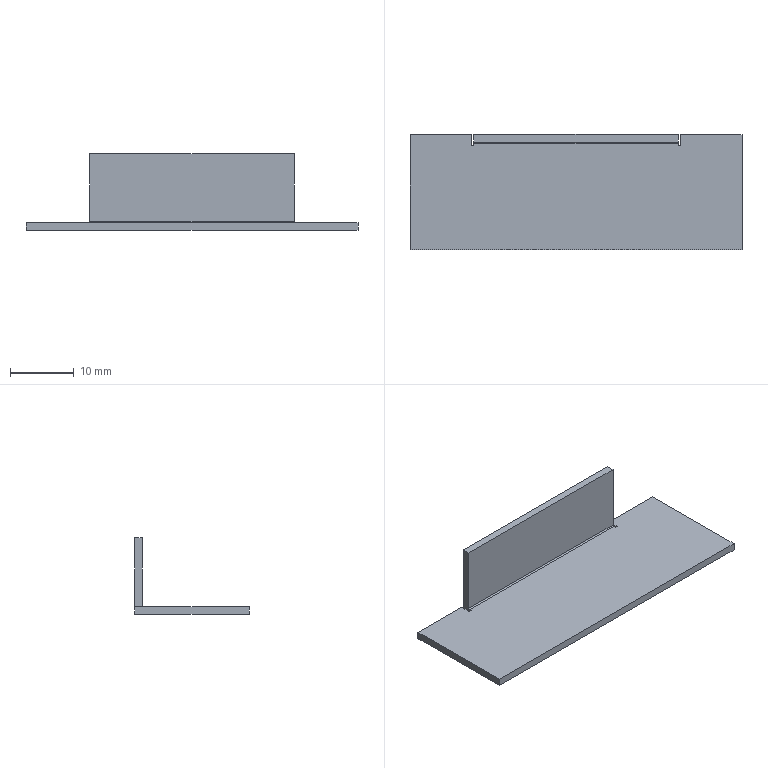Part | STEP file | FHD-021-007-C TZD10S drawer 3 | 1 solid | 18 faces | box 52 x 18 x 12 mm | volume 1523 mm3 | plane 16 | cylinder 2 | commonest cylinder face diameters 0.4 x1 2.8 x1
STEP:
#1=CARTESIAN_POINT('',(0.,0.,0.));
#2=DIRECTION('',(0.,0.,1.));
#3=DIRECTION('',(1.,0.,0.));
#4=AXIS2_PLACEMENT_3D('',#1,#2,#3);
#5=CARTESIAN_POINT('',(-16.,7.24,-1.2));
#6=VERTEX_POINT('',#5);
#7=CARTESIAN_POINT('',(-16.36,7.24,-1.2));
#8=VERTEX_POINT('',#7);
#9=CARTESIAN_POINT('',(0.,7.24,-1.2));
#10=DIRECTION('',(-1.,0.,0.));
#11=VECTOR('',#10,1.);
#12=LINE('',#9,#11);
#13=CARTESIAN_POINT('',(0.,0.,-1.2));
#14=DIRECTION('',(0.,0.,1.));
#15=DIRECTION('',(1.,0.,0.));
#16=AXIS2_PLACEMENT_3D('',#13,#14,#15);
#17=PLANE('',#16);
#18=CARTESIAN_POINT('',(0.,7.24));
#19=DIRECTION('',(-1.,0.));
#20=VECTOR('',#19,1.);
#21=LINE('',#18,#20);
#22=(GEOMETRIC_REPRESENTATION_CONTEXT(2)PARAMETRIC_REPRESENTATION_CONTEXT()REPRESENTATION_CONTEXT('',''));
#23=DEFINITIONAL_REPRESENTATION('',(#21),#22);
#24=PCURVE('',#17,#23);
#25=CARTESIAN_POINT('',(-16.36,7.24,0.));
#26=DIRECTION('',(0.,1.,0.));
#27=DIRECTION('',(0.,0.,1.));
#28=AXIS2_PLACEMENT_3D('',#25,#26,#27);
#29=PLANE('',#28);
#30=CARTESIAN_POINT('',(-1.2,16.36));
#31=DIRECTION('',(0.,-1.));
#32=VECTOR('',#31,1.);
#33=LINE('',#30,#32);
#34=(GEOMETRIC_REPRESENTATION_CONTEXT(2)PARAMETRIC_REPRESENTATION_CONTEXT()REPRESENTATION_CONTEXT('',''));
#35=DEFINITIONAL_REPRESENTATION('',(#33),#34);
#36=PCURVE('',#29,#35);
#37=SURFACE_CURVE('',#12,(#24,#36),.PCURVE_S1.);
#38=EDGE_CURVE('',#6,#8,#37,.T.);
#39=ORIENTED_EDGE('',*,*,#38,.F.);
#40=CARTESIAN_POINT('',(-16.,7.6,-1.2));
#41=VERTEX_POINT('',#40);
#42=CARTESIAN_POINT('',(-16.,0.,-1.2));
#43=DIRECTION('',(0.,-1.,0.));
#44=VECTOR('',#43,1.);
#45=LINE('',#42,#44);
#46=CARTESIAN_POINT('',(-16.,0.));
#47=DIRECTION('',(0.,-1.));
#48=VECTOR('',#47,1.);
#49=LINE('',#46,#48);
#50=(GEOMETRIC_REPRESENTATION_CONTEXT(2)PARAMETRIC_REPRESENTATION_CONTEXT()REPRESENTATION_CONTEXT('',''));
#51=DEFINITIONAL_REPRESENTATION('',(#49),#50);
#52=PCURVE('',#17,#51);
#53=CARTESIAN_POINT('',(-16.,7.24,0.));
#54=DIRECTION('',(-1.,0.,0.));
#55=DIRECTION('',(0.,0.,1.));
#56=AXIS2_PLACEMENT_3D('',#53,#54,#55);
#57=PLANE('',#56);
#58=CARTESIAN_POINT('',(-1.2,-7.24));
#59=DIRECTION('',(0.,-1.));
#60=VECTOR('',#59,1.);
#61=LINE('',#58,#60);
#62=(GEOMETRIC_REPRESENTATION_CONTEXT(2)PARAMETRIC_REPRESENTATION_CONTEXT()REPRESENTATION_CONTEXT('',''));
#63=DEFINITIONAL_REPRESENTATION('',(#61),#62);
#64=PCURVE('',#57,#63);
#65=SURFACE_CURVE('',#45,(#52,#64),.PCURVE_S1.);
#66=EDGE_CURVE('',#41,#6,#65,.T.);
#67=ORIENTED_EDGE('',*,*,#66,.F.);
#68=CARTESIAN_POINT('',(16.,7.6,-1.2));
#69=VERTEX_POINT('',#68);
#70=CARTESIAN_POINT('',(0.,7.6,-1.2));
#71=DIRECTION('',(-1.,0.,0.));
#72=VECTOR('',#71,1.);
#73=LINE('',#70,#72);
#74=CARTESIAN_POINT('',(0.,7.6));
#75=DIRECTION('',(-1.,0.));
#76=VECTOR('',#75,1.);
#77=LINE('',#74,#76);
#78=(GEOMETRIC_REPRESENTATION_CONTEXT(2)PARAMETRIC_REPRESENTATION_CONTEXT()REPRESENTATION_CONTEXT('',''));
#79=DEFINITIONAL_REPRESENTATION('',(#77),#78);
#80=PCURVE('',#17,#79);
#81=CARTESIAN_POINT('',(-16.,7.6,0.2));
#82=DIRECTION('',(-1.,0.,0.));
#83=DIRECTION('',(0.,0.,1.));
#84=AXIS2_PLACEMENT_3D('',#81,#82,#83);
#85=CYLINDRICAL_SURFACE('',#84,1.4);
#86=CARTESIAN_POINT('',(3.142,-16.));
#87=DIRECTION('',(0.,1.));
#88=VECTOR('',#87,1.);
#89=LINE('',#86,#88);
#90=(GEOMETRIC_REPRESENTATION_CONTEXT(2)PARAMETRIC_REPRESENTATION_CONTEXT()REPRESENTATION_CONTEXT('',''));
#91=DEFINITIONAL_REPRESENTATION('',(#89),#90);
#92=PCURVE('',#85,#91);
#93=SURFACE_CURVE('',#73,(#80,#92),.PCURVE_S1.);
#94=EDGE_CURVE('',#69,#41,#93,.T.);
#95=ORIENTED_EDGE('',*,*,#94,.F.);
#96=CARTESIAN_POINT('',(16.,7.24,-1.2));
#97=VERTEX_POINT('',#96);
#98=CARTESIAN_POINT('',(16.,0.,-1.2));
#99=DIRECTION('',(0.,1.,0.));
#100=VECTOR('',#99,1.);
#101=LINE('',#98,#100);
#102=CARTESIAN_POINT('',(16.,0.));
#103=DIRECTION('',(0.,1.));
#104=VECTOR('',#103,1.);
#105=LINE('',#102,#104);
#106=(GEOMETRIC_REPRESENTATION_CONTEXT(2)PARAMETRIC_REPRESENTATION_CONTEXT()REPRESENTATION_CONTEXT('',''));
#107=DEFINITIONAL_REPRESENTATION('',(#105),#106);
#108=PCURVE('',#17,#107);
#109=CARTESIAN_POINT('',(16.,7.6,0.));
#110=DIRECTION('',(1.,0.,0.));
#111=DIRECTION('',(0.,0.,-1.));
#112=AXIS2_PLACEMENT_3D('',#109,#110,#111);
#113=PLANE('',#112);
#114=CARTESIAN_POINT('',(1.2,-7.6));
#115=DIRECTION('',(0.,1.));
#116=VECTOR('',#115,1.);
#117=LINE('',#114,#116);
#118=(GEOMETRIC_REPRESENTATION_CONTEXT(2)PARAMETRIC_REPRESENTATION_CONTEXT()REPRESENTATION_CONTEXT('',''));
#119=DEFINITIONAL_REPRESENTATION('',(#117),#118);
#120=PCURVE('',#113,#119);
#121=SURFACE_CURVE('',#101,(#108,#120),.PCURVE_S1.);
#122=EDGE_CURVE('',#97,#69,#121,.T.);
#123=ORIENTED_EDGE('',*,*,#122,.F.);
#124=CARTESIAN_POINT('',(16.36,7.24,-1.2));
#125=VERTEX_POINT('',#124);
#126=CARTESIAN_POINT('',(0.,7.24,-1.2));
#127=DIRECTION('',(-1.,0.,0.));
#128=VECTOR('',#127,1.);
#129=LINE('',#126,#128);
#130=CARTESIAN_POINT('',(0.,7.24));
#131=DIRECTION('',(-1.,0.));
#132=VECTOR('',#131,1.);
#133=LINE('',#130,#132);
#134=(GEOMETRIC_REPRESENTATION_CONTEXT(2)PARAMETRIC_REPRESENTATION_CONTEXT()REPRESENTATION_CONTEXT('',''));
#135=DEFINITIONAL_REPRESENTATION('',(#133),#134);
#136=PCURVE('',#17,#135);
#137=CARTESIAN_POINT('',(16.,7.24,0.));
#138=DIRECTION('',(0.,1.,0.));
#139=DIRECTION('',(0.,0.,1.));
#140=AXIS2_PLACEMENT_3D('',#137,#138,#139);
#141=PLANE('',#140);
#142=CARTESIAN_POINT('',(-1.2,-16.));
#143=DIRECTION('',(0.,-1.));
#144=VECTOR('',#143,1.);
#145=LINE('',#142,#144);
#146=(GEOMETRIC_REPRESENTATION_CONTEXT(2)PARAMETRIC_REPRESENTATION_CONTEXT()REPRESENTATION_CONTEXT('',''));
#147=DEFINITIONAL_REPRESENTATION('',(#145),#146);
#148=PCURVE('',#141,#147);
#149=SURFACE_CURVE('',#129,(#136,#148),.PCURVE_S1.);
#150=EDGE_CURVE('',#125,#97,#149,.T.);
#151=ORIENTED_EDGE('',*,*,#150,.F.);
#152=CARTESIAN_POINT('',(16.36,9.,-1.2));
#153=VERTEX_POINT('',#152);
#154=CARTESIAN_POINT('',(16.36,0.,-1.2));
#155=DIRECTION('',(0.,-1.,0.));
#156=VECTOR('',#155,1.);
#157=LINE('',#154,#156);
#158=CARTESIAN_POINT('',(16.36,0.));
#159=DIRECTION('',(0.,-1.));
#160=VECTOR('',#159,1.);
#161=LINE('',#158,#160);
#162=(GEOMETRIC_REPRESENTATION_CONTEXT(2)PARAMETRIC_REPRESENTATION_CONTEXT()REPRESENTATION_CONTEXT('',''));
#163=DEFINITIONAL_REPRESENTATION('',(#161),#162);
#164=PCURVE('',#17,#163);
#165=CARTESIAN_POINT('',(16.36,7.24,0.));
#166=DIRECTION('',(-1.,0.,0.));
#167=DIRECTION('',(0.,-1.,0.));
#168=AXIS2_PLACEMENT_3D('',#165,#166,#167);
#169=PLANE('',#168);
#170=CARTESIAN_POINT('',(7.24,-1.2));
#171=DIRECTION('',(1.,0.));
#172=VECTOR('',#171,1.);
#173=LINE('',#170,#172);
#174=(GEOMETRIC_REPRESENTATION_CONTEXT(2)PARAMETRIC_REPRESENTATION_CONTEXT()REPRESENTATION_CONTEXT('',''));
#175=DEFINITIONAL_REPRESENTATION('',(#173),#174);
#176=PCURVE('',#169,#175);
#177=SURFACE_CURVE('',#157,(#164,#176),.PCURVE_S1.);
#178=EDGE_CURVE('',#153,#125,#177,.T.);
#179=ORIENTED_EDGE('',*,*,#178,.F.);
#180=CARTESIAN_POINT('',(26.,9.,-1.2));
#181=VERTEX_POINT('',#180);
#182=CARTESIAN_POINT('',(0.,9.,-1.2));
#183=DIRECTION('',(-1.,0.,0.));
#184=VECTOR('',#183,1.);
#185=LINE('',#182,#184);
#186=CARTESIAN_POINT('',(0.,9.));
#187=DIRECTION('',(-1.,0.));
#188=VECTOR('',#187,1.);
#189=LINE('',#186,#188);
#190=(GEOMETRIC_REPRESENTATION_CONTEXT(2)PARAMETRIC_REPRESENTATION_CONTEXT()REPRESENTATION_CONTEXT('',''));
#191=DEFINITIONAL_REPRESENTATION('',(#189),#190);
#192=PCURVE('',#17,#191);
#193=CARTESIAN_POINT('',(-26.,9.,-1.2));
#194=DIRECTION('',(0.,1.,0.));
#195=DIRECTION('',(0.,0.,1.));
#196=AXIS2_PLACEMENT_3D('',#193,#194,#195);
#197=PLANE('',#196);
#198=CARTESIAN_POINT('',(0.,26.));
#199=DIRECTION('',(0.,-1.));
#200=VECTOR('',#199,1.);
#201=LINE('',#198,#200);
#202=(GEOMETRIC_REPRESENTATION_CONTEXT(2)PARAMETRIC_REPRESENTATION_CONTEXT()REPRESENTATION_CONTEXT('',''));
#203=DEFINITIONAL_REPRESENTATION('',(#201),#202);
#204=PCURVE('',#197,#203);
#205=SURFACE_CURVE('',#185,(#192,#204),.PCURVE_S1.);
#206=EDGE_CURVE('',#181,#153,#205,.T.);
#207=ORIENTED_EDGE('',*,*,#206,.F.);
#208=CARTESIAN_POINT('',(26.,-9.,-1.2));
#209=VERTEX_POINT('',#208);
#210=CARTESIAN_POINT('',(26.,0.,-1.2));
#211=DIRECTION('',(0.,1.,0.));
#212=VECTOR('',#211,1.);
#213=LINE('',#210,#212);
#214=CARTESIAN_POINT('',(26.,0.));
#215=DIRECTION('',(0.,1.));
#216=VECTOR('',#215,1.);
#217=LINE('',#214,#216);
#218=(GEOMETRIC_REPRESENTATION_CONTEXT(2)PARAMETRIC_REPRESENTATION_CONTEXT()REPRESENTATION_CONTEXT('',''));
#219=DEFINITIONAL_REPRESENTATION('',(#217),#218);
#220=PCURVE('',#17,#219);
#221=CARTESIAN_POINT('',(26.,9.,-1.2));
#222=DIRECTION('',(1.,0.,0.));
#223=DIRECTION('',(0.,0.,-1.));
#224=AXIS2_PLACEMENT_3D('',#221,#222,#223);
#225=PLANE('',#224);
#226=CARTESIAN_POINT('',(0.,-9.));
#227=DIRECTION('',(0.,1.));
#228=VECTOR('',#227,1.);
#229=LINE('',#226,#228);
#230=(GEOMETRIC_REPRESENTATION_CONTEXT(2)PARAMETRIC_REPRESENTATION_CONTEXT()REPRESENTATION_CONTEXT('',''));
#231=DEFINITIONAL_REPRESENTATION('',(#229),#230);
#232=PCURVE('',#225,#231);
#233=SURFACE_CURVE('',#213,(#220,#232),.PCURVE_S1.);
#234=EDGE_CURVE('',#209,#181,#233,.T.);
#235=ORIENTED_EDGE('',*,*,#234,.F.);
#236=CARTESIAN_POINT('',(-26.,-9.,-1.2));
#237=VERTEX_POINT('',#236);
#238=CARTESIAN_POINT('',(0.,-9.,-1.2));
#239=DIRECTION('',(1.,0.,0.));
#240=VECTOR('',#239,1.);
#241=LINE('',#238,#240);
#242=CARTESIAN_POINT('',(0.,-9.));
#243=DIRECTION('',(1.,0.));
#244=VECTOR('',#243,1.);
#245=LINE('',#242,#244);
#246=(GEOMETRIC_REPRESENTATION_CONTEXT(2)PARAMETRIC_REPRESENTATION_CONTEXT()REPRESENTATION_CONTEXT('',''));
#247=DEFINITIONAL_REPRESENTATION('',(#245),#246);
#248=PCURVE('',#17,#247);
#249=CARTESIAN_POINT('',(-26.,-9.,-1.2));
#250=DIRECTION('',(0.,-1.,0.));
#251=DIRECTION('',(0.,0.,-1.));
#252=AXIS2_PLACEMENT_3D('',#249,#250,#251);
#253=PLANE('',#252);
#254=CARTESIAN_POINT('',(0.,26.));
#255=DIRECTION('',(0.,1.));
#256=VECTOR('',#255,1.);
#257=LINE('',#254,#256);
#258=(GEOMETRIC_REPRESENTATION_CONTEXT(2)PARAMETRIC_REPRESENTATION_CONTEXT()REPRESENTATION_CONTEXT('',''));
#259=DEFINITIONAL_REPRESENTATION('',(#257),#258);
#260=PCURVE('',#253,#259);
#261=SURFACE_CURVE('',#241,(#248,#260),.PCURVE_S1.);
#262=EDGE_CURVE('',#237,#209,#261,.T.);
#263=ORIENTED_EDGE('',*,*,#262,.F.);
#264=CARTESIAN_POINT('',(-26.,9.,-1.2));
#265=VERTEX_POINT('',#264);
#266=CARTESIAN_POINT('',(-26.,0.,-1.2));
#267=DIRECTION('',(0.,-1.,0.));
#268=VECTOR('',#267,1.);
#269=LINE('',#266,#268);
#270=CARTESIAN_POINT('',(-26.,0.));
#271=DIRECTION('',(0.,-1.));
#272=VECTOR('',#271,1.);
#273=LINE('',#270,#272);
#274=(GEOMETRIC_REPRESENTATION_CONTEXT(2)PARAMETRIC_REPRESENTATION_CONTEXT()REPRESENTATION_CONTEXT('',''));
#275=DEFINITIONAL_REPRESENTATION('',(#273),#274);
#276=PCURVE('',#17,#275);
#277=CARTESIAN_POINT('',(-26.,9.,-1.2));
#278=DIRECTION('',(-1.,0.,0.));
#279=DIRECTION('',(0.,-1.,0.));
#280=AXIS2_PLACEMENT_3D('',#277,#278,#279);
#281=PLANE('',#280);
#282=CARTESIAN_POINT('',(9.,0.));
#283=DIRECTION('',(1.,0.));
#284=VECTOR('',#283,1.);
#285=LINE('',#282,#284);
#286=(GEOMETRIC_REPRESENTATION_CONTEXT(2)PARAMETRIC_REPRESENTATION_CONTEXT()REPRESENTATION_CONTEXT('',''));
#287=DEFINITIONAL_REPRESENTATION('',(#285),#286);
#288=PCURVE('',#281,#287);
#289=SURFACE_CURVE('',#269,(#276,#288),.PCURVE_S1.);
#290=EDGE_CURVE('',#265,#237,#289,.T.);
#291=ORIENTED_EDGE('',*,*,#290,.F.);
#292=CARTESIAN_POINT('',(-16.36,9.,-1.2));
#293=VERTEX_POINT('',#292);
#294=CARTESIAN_POINT('',(0.,9.,-1.2));
#295=DIRECTION('',(-1.,0.,0.));
#296=VECTOR('',#295,1.);
#297=LINE('',#294,#296);
#298=CARTESIAN_POINT('',(0.,9.));
#299=DIRECTION('',(-1.,0.));
#300=VECTOR('',#299,1.);
#301=LINE('',#298,#300);
#302=(GEOMETRIC_REPRESENTATION_CONTEXT(2)PARAMETRIC_REPRESENTATION_CONTEXT()REPRESENTATION_CONTEXT('',''));
#303=DEFINITIONAL_REPRESENTATION('',(#301),#302);
#304=PCURVE('',#17,#303);
#305=CARTESIAN_POINT('',(-26.,9.,-1.2));
#306=DIRECTION('',(0.,1.,0.));
#307=DIRECTION('',(0.,0.,1.));
#308=AXIS2_PLACEMENT_3D('',#305,#306,#307);
#309=PLANE('',#308);
#310=CARTESIAN_POINT('',(0.,26.));
#311=DIRECTION('',(0.,-1.));
#312=VECTOR('',#311,1.);
#313=LINE('',#310,#312);
#314=(GEOMETRIC_REPRESENTATION_CONTEXT(2)PARAMETRIC_REPRESENTATION_CONTEXT()REPRESENTATION_CONTEXT('',''));
#315=DEFINITIONAL_REPRESENTATION('',(#313),#314);
#316=PCURVE('',#309,#315);
#317=SURFACE_CURVE('',#297,(#304,#316),.PCURVE_S1.);
#318=EDGE_CURVE('',#293,#265,#317,.T.);
#319=ORIENTED_EDGE('',*,*,#318,.F.);
#320=CARTESIAN_POINT('',(-16.36,0.,-1.2));
#321=DIRECTION('',(0.,1.,0.));
#322=VECTOR('',#321,1.);
#323=LINE('',#320,#322);
#324=CARTESIAN_POINT('',(-16.36,0.));
#325=DIRECTION('',(0.,1.));
#326=VECTOR('',#325,1.);
#327=LINE('',#324,#326);
#328=(GEOMETRIC_REPRESENTATION_CONTEXT(2)PARAMETRIC_REPRESENTATION_CONTEXT()REPRESENTATION_CONTEXT('',''));
#329=DEFINITIONAL_REPRESENTATION('',(#327),#328);
#330=PCURVE('',#17,#329);
#331=CARTESIAN_POINT('',(-16.36,9.,0.));
#332=DIRECTION('',(1.,0.,0.));
#333=DIRECTION('',(0.,0.,-1.));
#334=AXIS2_PLACEMENT_3D('',#331,#332,#333);
#335=PLANE('',#334);
#336=CARTESIAN_POINT('',(1.2,-9.));
#337=DIRECTION('',(0.,1.));
#338=VECTOR('',#337,1.);
#339=LINE('',#336,#338);
#340=(GEOMETRIC_REPRESENTATION_CONTEXT(2)PARAMETRIC_REPRESENTATION_CONTEXT()REPRESENTATION_CONTEXT('',''));
#341=DEFINITIONAL_REPRESENTATION('',(#339),#340);
#342=PCURVE('',#335,#341);
#343=SURFACE_CURVE('',#323,(#330,#342),.PCURVE_S1.);
#344=EDGE_CURVE('',#8,#293,#343,.T.);
#345=ORIENTED_EDGE('',*,*,#344,.F.);
#346=EDGE_LOOP('',(#39,#67,#95,#123,#151,#179,#207,#235,#263,#291,#319,#345));
#347=FACE_BOUND('',#346,.T.);
#348=ADVANCED_FACE('',(#347),#17,.F.);
#349=CARTESIAN_POINT('',(-16.36,9.,0.));
#350=VERTEX_POINT('',#349);
#351=CARTESIAN_POINT('',(-16.36,9.,0.));
#352=DIRECTION('',(0.,0.,1.));
#353=VECTOR('',#352,1.);
#354=LINE('',#351,#353);
#355=CARTESIAN_POINT('',(0.,0.));
#356=DIRECTION('',(-1.,0.));
#357=VECTOR('',#356,1.);
#358=LINE('',#355,#357);
#359=(GEOMETRIC_REPRESENTATION_CONTEXT(2)PARAMETRIC_REPRESENTATION_CONTEXT()REPRESENTATION_CONTEXT('',''));
#360=DEFINITIONAL_REPRESENTATION('',(#358),#359);
#361=PCURVE('',#335,#360);
#362=CARTESIAN_POINT('',(1.2,9.64));
#363=DIRECTION('',(1.,0.));
#364=VECTOR('',#363,1.);
#365=LINE('',#362,#364);
#366=(GEOMETRIC_REPRESENTATION_CONTEXT(2)PARAMETRIC_REPRESENTATION_CONTEXT()REPRESENTATION_CONTEXT('',''));
#367=DEFINITIONAL_REPRESENTATION('',(#365),#366);
#368=PCURVE('',#309,#367);
#369=SURFACE_CURVE('',#354,(#361,#368),.PCURVE_S1.);
#370=EDGE_CURVE('',#293,#350,#369,.T.);
#371=ORIENTED_EDGE('',*,*,#370,.T.);
#372=CARTESIAN_POINT('',(-16.36,7.24,0.));
#373=VERTEX_POINT('',#372);
#374=CARTESIAN_POINT('',(-16.36,9.,0.));
#375=DIRECTION('',(0.,-1.,0.));
#376=VECTOR('',#375,1.);
#377=LINE('',#374,#376);
#378=CARTESIAN_POINT('',(0.,0.));
#379=DIRECTION('',(0.,-1.));
#380=VECTOR('',#379,1.);
#381=LINE('',#378,#380);
#382=(GEOMETRIC_REPRESENTATION_CONTEXT(2)PARAMETRIC_REPRESENTATION_CONTEXT()REPRESENTATION_CONTEXT('',''));
#383=DEFINITIONAL_REPRESENTATION('',(#381),#382);
#384=PCURVE('',#335,#383);
#385=CARTESIAN_POINT('',(0.,0.,0.));
#386=DIRECTION('',(0.,0.,1.));
#387=DIRECTION('',(1.,0.,0.));
#388=AXIS2_PLACEMENT_3D('',#385,#386,#387);
#389=PLANE('',#388);
#390=CARTESIAN_POINT('',(-16.36,9.));
#391=DIRECTION('',(0.,-1.));
#392=VECTOR('',#391,1.);
#393=LINE('',#390,#392);
#394=(GEOMETRIC_REPRESENTATION_CONTEXT(2)PARAMETRIC_REPRESENTATION_CONTEXT()REPRESENTATION_CONTEXT('',''));
#395=DEFINITIONAL_REPRESENTATION('',(#393),#394);
#396=PCURVE('',#389,#395);
#397=SURFACE_CURVE('',#377,(#384,#396),.PCURVE_S1.);
#398=EDGE_CURVE('',#350,#373,#397,.T.);
#399=ORIENTED_EDGE('',*,*,#398,.T.);
#400=CARTESIAN_POINT('',(-16.36,7.24,0.));
#401=DIRECTION('',(0.,0.,-1.));
#402=VECTOR('',#401,1.);
#403=LINE('',#400,#402);
#404=CARTESIAN_POINT('',(0.,-1.76));
#405=DIRECTION('',(1.,0.));
#406=VECTOR('',#405,1.);
#407=LINE('',#404,#406);
#408=(GEOMETRIC_REPRESENTATION_CONTEXT(2)PARAMETRIC_REPRESENTATION_CONTEXT()REPRESENTATION_CONTEXT('',''));
#409=DEFINITIONAL_REPRESENTATION('',(#407),#408);
#410=PCURVE('',#335,#409);
#411=CARTESIAN_POINT('',(0.,0.));
#412=DIRECTION('',(-1.,0.));
#413=VECTOR('',#412,1.);
#414=LINE('',#411,#413);
#415=(GEOMETRIC_REPRESENTATION_CONTEXT(2)PARAMETRIC_REPRESENTATION_CONTEXT()REPRESENTATION_CONTEXT('',''));
#416=DEFINITIONAL_REPRESENTATION('',(#414),#415);
#417=PCURVE('',#29,#416);
#418=SURFACE_CURVE('',#403,(#410,#417),.PCURVE_S1.);
#419=EDGE_CURVE('',#373,#8,#418,.T.);
#420=ORIENTED_EDGE('',*,*,#419,.T.);
#421=ORIENTED_EDGE('',*,*,#344,.T.);
#422=EDGE_LOOP('',(#371,#399,#420,#421));
#423=FACE_BOUND('',#422,.T.);
#424=ADVANCED_FACE('',(#423),#335,.T.);
#425=ORIENTED_EDGE('',*,*,#419,.F.);
#426=CARTESIAN_POINT('',(-16.,7.24,0.));
#427=VERTEX_POINT('',#426);
#428=CARTESIAN_POINT('',(-16.36,7.24,0.));
#429=DIRECTION('',(1.,0.,0.));
#430=VECTOR('',#429,1.);
#431=LINE('',#428,#430);
#432=CARTESIAN_POINT('',(0.,0.));
#433=DIRECTION('',(0.,1.));
#434=VECTOR('',#433,1.);
#435=LINE('',#432,#434);
#436=(GEOMETRIC_REPRESENTATION_CONTEXT(2)PARAMETRIC_REPRESENTATION_CONTEXT()REPRESENTATION_CONTEXT('',''));
#437=DEFINITIONAL_REPRESENTATION('',(#435),#436);
#438=PCURVE('',#29,#437);
#439=CARTESIAN_POINT('',(-16.36,7.24));
#440=DIRECTION('',(1.,0.));
#441=VECTOR('',#440,1.);
#442=LINE('',#439,#441);
#443=(GEOMETRIC_REPRESENTATION_CONTEXT(2)PARAMETRIC_REPRESENTATION_CONTEXT()REPRESENTATION_CONTEXT('',''));
#444=DEFINITIONAL_REPRESENTATION('',(#442),#443);
#445=PCURVE('',#389,#444);
#446=SURFACE_CURVE('',#431,(#438,#445),.PCURVE_S1.);
#447=EDGE_CURVE('',#373,#427,#446,.T.);
#448=ORIENTED_EDGE('',*,*,#447,.T.);
#449=CARTESIAN_POINT('',(-16.,7.24,0.));
#450=DIRECTION('',(0.,0.,-1.));
#451=VECTOR('',#450,1.);
#452=LINE('',#449,#451);
#453=CARTESIAN_POINT('',(0.,0.36));
#454=DIRECTION('',(-1.,0.));
#455=VECTOR('',#454,1.);
#456=LINE('',#453,#455);
#457=(GEOMETRIC_REPRESENTATION_CONTEXT(2)PARAMETRIC_REPRESENTATION_CONTEXT()REPRESENTATION_CONTEXT('',''));
#458=DEFINITIONAL_REPRESENTATION('',(#456),#457);
#459=PCURVE('',#29,#458);
#460=CARTESIAN_POINT('',(0.,0.));
#461=DIRECTION('',(-1.,0.));
#462=VECTOR('',#461,1.);
#463=LINE('',#460,#462);
#464=(GEOMETRIC_REPRESENTATION_CONTEXT(2)PARAMETRIC_REPRESENTATION_CONTEXT()REPRESENTATION_CONTEXT('',''));
#465=DEFINITIONAL_REPRESENTATION('',(#463),#464);
#466=PCURVE('',#57,#465);
#467=SURFACE_CURVE('',#452,(#459,#466),.PCURVE_S1.);
#468=EDGE_CURVE('',#427,#6,#467,.T.);
#469=ORIENTED_EDGE('',*,*,#468,.T.);
#470=ORIENTED_EDGE('',*,*,#38,.T.);
#471=EDGE_LOOP('',(#425,#448,#469,#470));
#472=FACE_BOUND('',#471,.T.);
#473=ADVANCED_FACE('',(#472),#29,.T.);
#474=ORIENTED_EDGE('',*,*,#468,.F.);
#475=CARTESIAN_POINT('',(-16.,7.6,0.));
#476=VERTEX_POINT('',#475);
#477=CARTESIAN_POINT('',(-16.,7.24,0.));
#478=DIRECTION('',(0.,1.,0.));
#479=VECTOR('',#478,1.);
#480=LINE('',#477,#479);
#481=CARTESIAN_POINT('',(0.,0.));
#482=DIRECTION('',(0.,1.));
#483=VECTOR('',#482,1.);
#484=LINE('',#481,#483);
#485=(GEOMETRIC_REPRESENTATION_CONTEXT(2)PARAMETRIC_REPRESENTATION_CONTEXT()REPRESENTATION_CONTEXT('',''));
#486=DEFINITIONAL_REPRESENTATION('',(#484),#485);
#487=PCURVE('',#57,#486);
#488=CARTESIAN_POINT('',(-16.,7.24));
#489=DIRECTION('',(0.,1.));
#490=VECTOR('',#489,1.);
#491=LINE('',#488,#490);
#492=(GEOMETRIC_REPRESENTATION_CONTEXT(2)PARAMETRIC_REPRESENTATION_CONTEXT()REPRESENTATION_CONTEXT('',''));
#493=DEFINITIONAL_REPRESENTATION('',(#491),#492);
#494=PCURVE('',#389,#493);
#495=SURFACE_CURVE('',#480,(#487,#494),.PCURVE_S1.);
#496=EDGE_CURVE('',#427,#476,#495,.T.);
#497=ORIENTED_EDGE('',*,*,#496,.T.);
#498=CARTESIAN_POINT('',(-16.,7.8,0.2));
#499=VERTEX_POINT('',#498);
#500=CARTESIAN_POINT('',(-16.,7.6,0.2));
#501=DIRECTION('',(-1.,0.,0.));
#502=DIRECTION('',(0.,0.,1.));
#503=AXIS2_PLACEMENT_3D('',#500,#501,#502);
#504=CIRCLE('',#503,0.2);
#505=CARTESIAN_POINT('',(0.2,0.36));
#506=DIRECTION('',(1.,0.));
#507=AXIS2_PLACEMENT_2D('',#505,#506);
#508=CIRCLE('',#507,0.2);
#509=(GEOMETRIC_REPRESENTATION_CONTEXT(2)PARAMETRIC_REPRESENTATION_CONTEXT()REPRESENTATION_CONTEXT('',''));
#510=DEFINITIONAL_REPRESENTATION('',(#508),#509);
#511=PCURVE('',#57,#510);
#512=CARTESIAN_POINT('',(-16.,7.6,0.2));
#513=DIRECTION('',(-1.,0.,0.));
#514=DIRECTION('',(0.,0.,1.));
#515=AXIS2_PLACEMENT_3D('',#512,#513,#514);
#516=CYLINDRICAL_SURFACE('',#515,0.2);
#517=CARTESIAN_POINT('',(0.,0.));
#518=DIRECTION('',(1.,0.));
#519=VECTOR('',#518,1.);
#520=LINE('',#517,#519);
#521=(GEOMETRIC_REPRESENTATION_CONTEXT(2)PARAMETRIC_REPRESENTATION_CONTEXT()REPRESENTATION_CONTEXT('',''));
#522=DEFINITIONAL_REPRESENTATION('',(#520),#521);
#523=PCURVE('',#516,#522);
#524=SURFACE_CURVE('',#504,(#511,#523),.PCURVE_S1.);
#525=EDGE_CURVE('',#499,#476,#524,.T.);
#526=ORIENTED_EDGE('',*,*,#525,.F.);
#527=CARTESIAN_POINT('',(-16.,7.8,10.8));
#528=VERTEX_POINT('',#527);
#529=CARTESIAN_POINT('',(-16.,7.8,10.8));
#530=DIRECTION('',(0.,0.,-1.));
#531=VECTOR('',#530,1.);
#532=LINE('',#529,#531);
#533=CARTESIAN_POINT('',(10.8,0.56));
#534=DIRECTION('',(-1.,0.));
#535=VECTOR('',#534,1.);
#536=LINE('',#533,#535);
#537=(GEOMETRIC_REPRESENTATION_CONTEXT(2)PARAMETRIC_REPRESENTATION_CONTEXT()REPRESENTATION_CONTEXT('',''));
#538=DEFINITIONAL_REPRESENTATION('',(#536),#537);
#539=PCURVE('',#57,#538);
#540=CARTESIAN_POINT('',(0.,7.8,0.));
#541=DIRECTION('',(0.,-1.,0.));
#542=DIRECTION('',(0.,0.,-1.));
#543=AXIS2_PLACEMENT_3D('',#540,#541,#542);
#544=PLANE('',#543);
#545=CARTESIAN_POINT('',(-10.8,-16.));
#546=DIRECTION('',(1.,0.));
#547=VECTOR('',#546,1.);
#548=LINE('',#545,#547);
#549=(GEOMETRIC_REPRESENTATION_CONTEXT(2)PARAMETRIC_REPRESENTATION_CONTEXT()REPRESENTATION_CONTEXT('',''));
#550=DEFINITIONAL_REPRESENTATION('',(#548),#549);
#551=PCURVE('',#544,#550);
#552=SURFACE_CURVE('',#532,(#539,#551),.PCURVE_S1.);
#553=EDGE_CURVE('',#528,#499,#552,.T.);
#554=ORIENTED_EDGE('',*,*,#553,.F.);
#555=CARTESIAN_POINT('',(-16.,9.,10.8));
#556=VERTEX_POINT('',#555);
#557=CARTESIAN_POINT('',(-16.,9.,10.8));
#558=DIRECTION('',(0.,-1.,0.));
#559=VECTOR('',#558,1.);
#560=LINE('',#557,#559);
#561=CARTESIAN_POINT('',(10.8,1.76));
#562=DIRECTION('',(0.,-1.));
#563=VECTOR('',#562,1.);
#564=LINE('',#561,#563);
#565=(GEOMETRIC_REPRESENTATION_CONTEXT(2)PARAMETRIC_REPRESENTATION_CONTEXT()REPRESENTATION_CONTEXT('',''));
#566=DEFINITIONAL_REPRESENTATION('',(#564),#565);
#567=PCURVE('',#57,#566);
#568=CARTESIAN_POINT('',(16.,9.,10.8));
#569=DIRECTION('',(0.,0.,-1.));
#570=DIRECTION('',(0.,1.,0.));
#571=AXIS2_PLACEMENT_3D('',#568,#569,#570);
#572=PLANE('',#571);
#573=CARTESIAN_POINT('',(0.,-32.));
#574=DIRECTION('',(-1.,0.));
#575=VECTOR('',#574,1.);
#576=LINE('',#573,#575);
#577=(GEOMETRIC_REPRESENTATION_CONTEXT(2)PARAMETRIC_REPRESENTATION_CONTEXT()REPRESENTATION_CONTEXT('',''));
#578=DEFINITIONAL_REPRESENTATION('',(#576),#577);
#579=PCURVE('',#572,#578);
#580=SURFACE_CURVE('',#560,(#567,#579),.PCURVE_S1.);
#581=EDGE_CURVE('',#556,#528,#580,.T.);
#582=ORIENTED_EDGE('',*,*,#581,.F.);
#583=CARTESIAN_POINT('',(-16.,9.,0.2));
#584=VERTEX_POINT('',#583);
#585=CARTESIAN_POINT('',(-16.,9.,0.));
#586=DIRECTION('',(0.,0.,-1.));
#587=VECTOR('',#586,1.);
#588=LINE('',#585,#587);
#589=CARTESIAN_POINT('',(0.,1.76));
#590=DIRECTION('',(-1.,0.));
#591=VECTOR('',#590,1.);
#592=LINE('',#589,#591);
#593=(GEOMETRIC_REPRESENTATION_CONTEXT(2)PARAMETRIC_REPRESENTATION_CONTEXT()REPRESENTATION_CONTEXT('',''));
#594=DEFINITIONAL_REPRESENTATION('',(#592),#593);
#595=PCURVE('',#57,#594);
#596=CARTESIAN_POINT('',(0.,9.,0.));
#597=DIRECTION('',(0.,-1.,0.));
#598=DIRECTION('',(0.,0.,-1.));
#599=AXIS2_PLACEMENT_3D('',#596,#597,#598);
#600=PLANE('',#599);
#601=CARTESIAN_POINT('',(0.,-16.));
#602=DIRECTION('',(1.,0.));
#603=VECTOR('',#602,1.);
#604=LINE('',#601,#603);
#605=(GEOMETRIC_REPRESENTATION_CONTEXT(2)PARAMETRIC_REPRESENTATION_CONTEXT()REPRESENTATION_CONTEXT('',''));
#606=DEFINITIONAL_REPRESENTATION('',(#604),#605);
#607=PCURVE('',#600,#606);
#608=SURFACE_CURVE('',#588,(#595,#607),.PCURVE_S1.);
#609=EDGE_CURVE('',#556,#584,#608,.T.);
#610=ORIENTED_EDGE('',*,*,#609,.T.);
#611=CARTESIAN_POINT('',(-16.,7.6,0.2));
#612=DIRECTION('',(1.,0.,0.));
#613=DIRECTION('',(0.,0.,1.));
#614=AXIS2_PLACEMENT_3D('',#611,#612,#613);
#615=CIRCLE('',#614,1.4);
#616=CARTESIAN_POINT('',(1.6,0.36));
#617=CARTESIAN_POINT('',(1.6,-2.065));
#618=CARTESIAN_POINT('',(-0.5,-0.8524));
#619=CARTESIAN_POINT('',(-2.6,0.36));
#620=CARTESIAN_POINT('',(-0.5,1.572));
#621=CARTESIAN_POINT('',(1.6,2.785));
#622=CARTESIAN_POINT('',(1.6,0.36));
#623=(BOUNDED_CURVE()B_SPLINE_CURVE(2,(#616,#617,#618,#619,#620,#621,#622),.UNSPECIFIED.,.T.,.F.)B_SPLINE_CURVE_WITH_KNOTS((1,2,2,2,2,1),(-2.094,0.,2.094,4.189,6.283,8.378),.UNSPECIFIED.)CURVE()GEOMETRIC_REPRESENTATION_ITEM()RATIONAL_B_SPLINE_CURVE((1.,0.5,1.,0.5,1.,0.5,1.))REPRESENTATION_ITEM(''));
#624=(GEOMETRIC_REPRESENTATION_CONTEXT(2)PARAMETRIC_REPRESENTATION_CONTEXT()REPRESENTATION_CONTEXT('',''));
#625=DEFINITIONAL_REPRESENTATION('',(#623),#624);
#626=PCURVE('',#57,#625);
#627=CARTESIAN_POINT('',(6.283,0.));
#628=DIRECTION('',(-1.,0.));
#629=VECTOR('',#628,1.);
#630=LINE('',#627,#629);
#631=(GEOMETRIC_REPRESENTATION_CONTEXT(2)PARAMETRIC_REPRESENTATION_CONTEXT()REPRESENTATION_CONTEXT('',''));
#632=DEFINITIONAL_REPRESENTATION('',(#630),#631);
#633=PCURVE('',#85,#632);
#634=SURFACE_CURVE('',#615,(#626,#633),.PCURVE_S1.);
#635=EDGE_CURVE('',#41,#584,#634,.T.);
#636=ORIENTED_EDGE('',*,*,#635,.F.);
#637=ORIENTED_EDGE('',*,*,#66,.T.);
#638=EDGE_LOOP('',(#474,#497,#526,#554,#582,#610,#636,#637));
#639=FACE_BOUND('',#638,.T.);
#640=ADVANCED_FACE('',(#639),#57,.T.);
#641=CARTESIAN_POINT('',(16.,9.,0.2));
#642=VERTEX_POINT('',#641);
#643=CARTESIAN_POINT('',(-16.,9.,0.2));
#644=DIRECTION('',(1.,0.,0.));
#645=VECTOR('',#644,1.);
#646=LINE('',#643,#645);
#647=CARTESIAN_POINT('',(1.571,0.));
#648=DIRECTION('',(0.,-1.));
#649=VECTOR('',#648,1.);
#650=LINE('',#647,#649);
#651=(GEOMETRIC_REPRESENTATION_CONTEXT(2)PARAMETRIC_REPRESENTATION_CONTEXT()REPRESENTATION_CONTEXT('',''));
#652=DEFINITIONAL_REPRESENTATION('',(#650),#651);
#653=PCURVE('',#85,#652);
#654=CARTESIAN_POINT('',(-0.2,-16.));
#655=DIRECTION('',(0.,1.));
#656=VECTOR('',#655,1.);
#657=LINE('',#654,#656);
#658=(GEOMETRIC_REPRESENTATION_CONTEXT(2)PARAMETRIC_REPRESENTATION_CONTEXT()REPRESENTATION_CONTEXT('',''));
#659=DEFINITIONAL_REPRESENTATION('',(#657),#658);
#660=PCURVE('',#600,#659);
#661=SURFACE_CURVE('',#646,(#653,#660),.PCURVE_S1.);
#662=EDGE_CURVE('',#584,#642,#661,.T.);
#663=ORIENTED_EDGE('',*,*,#662,.T.);
#664=CARTESIAN_POINT('',(16.,7.6,0.2));
#665=DIRECTION('',(-1.,0.,0.));
#666=DIRECTION('',(0.,0.,1.));
#667=AXIS2_PLACEMENT_3D('',#664,#665,#666);
#668=CIRCLE('',#667,1.4);
#669=CARTESIAN_POINT('',(0.,-32.));
#670=DIRECTION('',(1.,0.));
#671=VECTOR('',#670,1.);
#672=LINE('',#669,#671);
#673=(GEOMETRIC_REPRESENTATION_CONTEXT(2)PARAMETRIC_REPRESENTATION_CONTEXT()REPRESENTATION_CONTEXT('',''));
#674=DEFINITIONAL_REPRESENTATION('',(#672),#673);
#675=PCURVE('',#85,#674);
#676=CARTESIAN_POINT('',(-1.6,0.));
#677=CARTESIAN_POINT('',(-1.6,2.425));
#678=CARTESIAN_POINT('',(0.5,1.212));
#679=CARTESIAN_POINT('',(2.6,0.));
#680=CARTESIAN_POINT('',(0.5,-1.212));
#681=CARTESIAN_POINT('',(-1.6,-2.425));
#682=CARTESIAN_POINT('',(-1.6,0.));
#683=(BOUNDED_CURVE()B_SPLINE_CURVE(2,(#676,#677,#678,#679,#680,#681,#682),.UNSPECIFIED.,.T.,.F.)B_SPLINE_CURVE_WITH_KNOTS((1,2,2,2,2,1),(-2.094,0.,2.094,4.189,6.283,8.378),.UNSPECIFIED.)CURVE()GEOMETRIC_REPRESENTATION_ITEM()RATIONAL_B_SPLINE_CURVE((1.,0.5,1.,0.5,1.,0.5,1.))REPRESENTATION_ITEM(''));
#684=(GEOMETRIC_REPRESENTATION_CONTEXT(2)PARAMETRIC_REPRESENTATION_CONTEXT()REPRESENTATION_CONTEXT('',''));
#685=DEFINITIONAL_REPRESENTATION('',(#683),#684);
#686=PCURVE('',#113,#685);
#687=SURFACE_CURVE('',#668,(#675,#686),.PCURVE_S1.);
#688=EDGE_CURVE('',#642,#69,#687,.T.);
#689=ORIENTED_EDGE('',*,*,#688,.T.);
#690=ORIENTED_EDGE('',*,*,#94,.T.);
#691=ORIENTED_EDGE('',*,*,#635,.T.);
#692=EDGE_LOOP('',(#663,#689,#690,#691));
#693=FACE_BOUND('',#692,.T.);
#694=ADVANCED_FACE('',(#693),#85,.T.);
#695=ORIENTED_EDGE('',*,*,#122,.T.);
#696=ORIENTED_EDGE('',*,*,#688,.F.);
#697=CARTESIAN_POINT('',(16.,9.,10.8));
#698=VERTEX_POINT('',#697);
#699=CARTESIAN_POINT('',(16.,9.,0.));
#700=DIRECTION('',(0.,0.,1.));
#701=VECTOR('',#700,1.);
#702=LINE('',#699,#701);
#703=CARTESIAN_POINT('',(0.,1.4));
#704=DIRECTION('',(-1.,0.));
#705=VECTOR('',#704,1.);
#706=LINE('',#703,#705);
#707=(GEOMETRIC_REPRESENTATION_CONTEXT(2)PARAMETRIC_REPRESENTATION_CONTEXT()REPRESENTATION_CONTEXT('',''));
#708=DEFINITIONAL_REPRESENTATION('',(#706),#707);
#709=PCURVE('',#113,#708);
#710=CARTESIAN_POINT('',(0.,16.));
#711=DIRECTION('',(-1.,0.));
#712=VECTOR('',#711,1.);
#713=LINE('',#710,#712);
#714=(GEOMETRIC_REPRESENTATION_CONTEXT(2)PARAMETRIC_REPRESENTATION_CONTEXT()REPRESENTATION_CONTEXT('',''));
#715=DEFINITIONAL_REPRESENTATION('',(#713),#714);
#716=PCURVE('',#600,#715);
#717=SURFACE_CURVE('',#702,(#709,#716),.PCURVE_S1.);
#718=EDGE_CURVE('',#642,#698,#717,.T.);
#719=ORIENTED_EDGE('',*,*,#718,.T.);
#720=CARTESIAN_POINT('',(16.,7.8,10.8));
#721=VERTEX_POINT('',#720);
#722=CARTESIAN_POINT('',(16.,9.,10.8));
#723=DIRECTION('',(0.,-1.,0.));
#724=VECTOR('',#723,1.);
#725=LINE('',#722,#724);
#726=CARTESIAN_POINT('',(-10.8,1.4));
#727=DIRECTION('',(0.,-1.));
#728=VECTOR('',#727,1.);
#729=LINE('',#726,#728);
#730=(GEOMETRIC_REPRESENTATION_CONTEXT(2)PARAMETRIC_REPRESENTATION_CONTEXT()REPRESENTATION_CONTEXT('',''));
#731=DEFINITIONAL_REPRESENTATION('',(#729),#730);
#732=PCURVE('',#113,#731);
#733=CARTESIAN_POINT('',(0.,0.));
#734=DIRECTION('',(-1.,0.));
#735=VECTOR('',#734,1.);
#736=LINE('',#733,#735);
#737=(GEOMETRIC_REPRESENTATION_CONTEXT(2)PARAMETRIC_REPRESENTATION_CONTEXT()REPRESENTATION_CONTEXT('',''));
#738=DEFINITIONAL_REPRESENTATION('',(#736),#737);
#739=PCURVE('',#572,#738);
#740=SURFACE_CURVE('',#725,(#732,#739),.PCURVE_S1.);
#741=EDGE_CURVE('',#698,#721,#740,.T.);
#742=ORIENTED_EDGE('',*,*,#741,.T.);
#743=CARTESIAN_POINT('',(16.,7.8,0.2));
#744=VERTEX_POINT('',#743);
#745=CARTESIAN_POINT('',(16.,7.8,0.));
#746=DIRECTION('',(0.,0.,1.));
#747=VECTOR('',#746,1.);
#748=LINE('',#745,#747);
#749=CARTESIAN_POINT('',(0.,0.2));
#750=DIRECTION('',(-1.,0.));
#751=VECTOR('',#750,1.);
#752=LINE('',#749,#751);
#753=(GEOMETRIC_REPRESENTATION_CONTEXT(2)PARAMETRIC_REPRESENTATION_CONTEXT()REPRESENTATION_CONTEXT('',''));
#754=DEFINITIONAL_REPRESENTATION('',(#752),#753);
#755=PCURVE('',#113,#754);
#756=CARTESIAN_POINT('',(0.,16.));
#757=DIRECTION('',(-1.,0.));
#758=VECTOR('',#757,1.);
#759=LINE('',#756,#758);
#760=(GEOMETRIC_REPRESENTATION_CONTEXT(2)PARAMETRIC_REPRESENTATION_CONTEXT()REPRESENTATION_CONTEXT('',''));
#761=DEFINITIONAL_REPRESENTATION('',(#759),#760);
#762=PCURVE('',#544,#761);
#763=SURFACE_CURVE('',#748,(#755,#762),.PCURVE_S1.);
#764=EDGE_CURVE('',#744,#721,#763,.T.);
#765=ORIENTED_EDGE('',*,*,#764,.F.);
#766=CARTESIAN_POINT('',(16.,7.6,0.));
#767=VERTEX_POINT('',#766);
#768=CARTESIAN_POINT('',(16.,7.6,0.2));
#769=DIRECTION('',(-1.,0.,0.));
#770=DIRECTION('',(0.,0.,1.));
#771=AXIS2_PLACEMENT_3D('',#768,#769,#770);
#772=CIRCLE('',#771,0.2);
#773=CARTESIAN_POINT('',(-0.4,0.));
#774=CARTESIAN_POINT('',(-0.4,0.3464));
#775=CARTESIAN_POINT('',(-0.1,0.1732));
#776=CARTESIAN_POINT('',(0.2,0.));
#777=CARTESIAN_POINT('',(-0.1,-0.1732));
#778=CARTESIAN_POINT('',(-0.4,-0.3464));
#779=CARTESIAN_POINT('',(-0.4,0.));
#780=(BOUNDED_CURVE()B_SPLINE_CURVE(2,(#773,#774,#775,#776,#777,#778,#779),.UNSPECIFIED.,.T.,.F.)B_SPLINE_CURVE_WITH_KNOTS((1,2,2,2,2,1),(-2.094,0.,2.094,4.189,6.283,8.378),.UNSPECIFIED.)CURVE()GEOMETRIC_REPRESENTATION_ITEM()RATIONAL_B_SPLINE_CURVE((1.,0.5,1.,0.5,1.,0.5,1.))REPRESENTATION_ITEM(''));
#781=(GEOMETRIC_REPRESENTATION_CONTEXT(2)PARAMETRIC_REPRESENTATION_CONTEXT()REPRESENTATION_CONTEXT('',''));
#782=DEFINITIONAL_REPRESENTATION('',(#780),#781);
#783=PCURVE('',#113,#782);
#784=CARTESIAN_POINT('',(0.,-32.));
#785=DIRECTION('',(1.,0.));
#786=VECTOR('',#785,1.);
#787=LINE('',#784,#786);
#788=(GEOMETRIC_REPRESENTATION_CONTEXT(2)PARAMETRIC_REPRESENTATION_CONTEXT()REPRESENTATION_CONTEXT('',''));
#789=DEFINITIONAL_REPRESENTATION('',(#787),#788);
#790=PCURVE('',#516,#789);
#791=SURFACE_CURVE('',#772,(#783,#790),.PCURVE_S1.);
#792=EDGE_CURVE('',#744,#767,#791,.T.);
#793=ORIENTED_EDGE('',*,*,#792,.T.);
#794=CARTESIAN_POINT('',(16.,7.24,0.));
#795=VERTEX_POINT('',#794);
#796=CARTESIAN_POINT('',(16.,7.6,0.));
#797=DIRECTION('',(0.,-1.,0.));
#798=VECTOR('',#797,1.);
#799=LINE('',#796,#798);
#800=CARTESIAN_POINT('',(0.,0.));
#801=DIRECTION('',(0.,-1.));
#802=VECTOR('',#801,1.);
#803=LINE('',#800,#802);
#804=(GEOMETRIC_REPRESENTATION_CONTEXT(2)PARAMETRIC_REPRESENTATION_CONTEXT()REPRESENTATION_CONTEXT('',''));
#805=DEFINITIONAL_REPRESENTATION('',(#803),#804);
#806=PCURVE('',#113,#805);
#807=CARTESIAN_POINT('',(16.,7.6));
#808=DIRECTION('',(0.,-1.));
#809=VECTOR('',#808,1.);
#810=LINE('',#807,#809);
#811=(GEOMETRIC_REPRESENTATION_CONTEXT(2)PARAMETRIC_REPRESENTATION_CONTEXT()REPRESENTATION_CONTEXT('',''));
#812=DEFINITIONAL_REPRESENTATION('',(#810),#811);
#813=PCURVE('',#389,#812);
#814=SURFACE_CURVE('',#799,(#806,#813),.PCURVE_S1.);
#815=EDGE_CURVE('',#767,#795,#814,.T.);
#816=ORIENTED_EDGE('',*,*,#815,.T.);
#817=CARTESIAN_POINT('',(16.,7.24,0.));
#818=DIRECTION('',(0.,0.,-1.));
#819=VECTOR('',#818,1.);
#820=LINE('',#817,#819);
#821=CARTESIAN_POINT('',(0.,-0.36));
#822=DIRECTION('',(1.,0.));
#823=VECTOR('',#822,1.);
#824=LINE('',#821,#823);
#825=(GEOMETRIC_REPRESENTATION_CONTEXT(2)PARAMETRIC_REPRESENTATION_CONTEXT()REPRESENTATION_CONTEXT('',''));
#826=DEFINITIONAL_REPRESENTATION('',(#824),#825);
#827=PCURVE('',#113,#826);
#828=CARTESIAN_POINT('',(0.,0.));
#829=DIRECTION('',(-1.,0.));
#830=VECTOR('',#829,1.);
#831=LINE('',#828,#830);
#832=(GEOMETRIC_REPRESENTATION_CONTEXT(2)PARAMETRIC_REPRESENTATION_CONTEXT()REPRESENTATION_CONTEXT('',''));
#833=DEFINITIONAL_REPRESENTATION('',(#831),#832);
#834=PCURVE('',#141,#833);
#835=SURFACE_CURVE('',#820,(#827,#834),.PCURVE_S1.);
#836=EDGE_CURVE('',#795,#97,#835,.T.);
#837=ORIENTED_EDGE('',*,*,#836,.T.);
#838=EDGE_LOOP('',(#695,#696,#719,#742,#765,#793,#816,#837));
#839=FACE_BOUND('',#838,.T.);
#840=ADVANCED_FACE('',(#839),#113,.T.);
#841=ORIENTED_EDGE('',*,*,#836,.F.);
#842=CARTESIAN_POINT('',(16.36,7.24,0.));
#843=VERTEX_POINT('',#842);
#844=CARTESIAN_POINT('',(16.,7.24,0.));
#845=DIRECTION('',(1.,0.,0.));
#846=VECTOR('',#845,1.);
#847=LINE('',#844,#846);
#848=CARTESIAN_POINT('',(0.,0.));
#849=DIRECTION('',(0.,1.));
#850=VECTOR('',#849,1.);
#851=LINE('',#848,#850);
#852=(GEOMETRIC_REPRESENTATION_CONTEXT(2)PARAMETRIC_REPRESENTATION_CONTEXT()REPRESENTATION_CONTEXT('',''));
#853=DEFINITIONAL_REPRESENTATION('',(#851),#852);
#854=PCURVE('',#141,#853);
#855=CARTESIAN_POINT('',(16.,7.24));
#856=DIRECTION('',(1.,0.));
#857=VECTOR('',#856,1.);
#858=LINE('',#855,#857);
#859=(GEOMETRIC_REPRESENTATION_CONTEXT(2)PARAMETRIC_REPRESENTATION_CONTEXT()REPRESENTATION_CONTEXT('',''));
#860=DEFINITIONAL_REPRESENTATION('',(#858),#859);
#861=PCURVE('',#389,#860);
#862=SURFACE_CURVE('',#847,(#854,#861),.PCURVE_S1.);
#863=EDGE_CURVE('',#795,#843,#862,.T.);
#864=ORIENTED_EDGE('',*,*,#863,.T.);
#865=CARTESIAN_POINT('',(16.36,7.24,0.));
#866=DIRECTION('',(0.,0.,-1.));
#867=VECTOR('',#866,1.);
#868=LINE('',#865,#867);
#869=CARTESIAN_POINT('',(0.,0.36));
#870=DIRECTION('',(-1.,0.));
#871=VECTOR('',#870,1.);
#872=LINE('',#869,#871);
#873=(GEOMETRIC_REPRESENTATION_CONTEXT(2)PARAMETRIC_REPRESENTATION_CONTEXT()REPRESENTATION_CONTEXT('',''));
#874=DEFINITIONAL_REPRESENTATION('',(#872),#873);
#875=PCURVE('',#141,#874);
#876=CARTESIAN_POINT('',(0.,0.));
#877=DIRECTION('',(0.,-1.));
#878=VECTOR('',#877,1.);
#879=LINE('',#876,#878);
#880=(GEOMETRIC_REPRESENTATION_CONTEXT(2)PARAMETRIC_REPRESENTATION_CONTEXT()REPRESENTATION_CONTEXT('',''));
#881=DEFINITIONAL_REPRESENTATION('',(#879),#880);
#882=PCURVE('',#169,#881);
#883=SURFACE_CURVE('',#868,(#875,#882),.PCURVE_S1.);
#884=EDGE_CURVE('',#843,#125,#883,.T.);
#885=ORIENTED_EDGE('',*,*,#884,.T.);
#886=ORIENTED_EDGE('',*,*,#150,.T.);
#887=EDGE_LOOP('',(#841,#864,#885,#886));
#888=FACE_BOUND('',#887,.T.);
#889=ADVANCED_FACE('',(#888),#141,.T.);
#890=ORIENTED_EDGE('',*,*,#884,.F.);
#891=CARTESIAN_POINT('',(16.36,9.,0.));
#892=VERTEX_POINT('',#891);
#893=CARTESIAN_POINT('',(16.36,7.24,0.));
#894=DIRECTION('',(0.,1.,0.));
#895=VECTOR('',#894,1.);
#896=LINE('',#893,#895);
#897=CARTESIAN_POINT('',(0.,0.));
#898=DIRECTION('',(-1.,0.));
#899=VECTOR('',#898,1.);
#900=LINE('',#897,#899);
#901=(GEOMETRIC_REPRESENTATION_CONTEXT(2)PARAMETRIC_REPRESENTATION_CONTEXT()REPRESENTATION_CONTEXT('',''));
#902=DEFINITIONAL_REPRESENTATION('',(#900),#901);
#903=PCURVE('',#169,#902);
#904=CARTESIAN_POINT('',(16.36,7.24));
#905=DIRECTION('',(0.,1.));
#906=VECTOR('',#905,1.);
#907=LINE('',#904,#906);
#908=(GEOMETRIC_REPRESENTATION_CONTEXT(2)PARAMETRIC_REPRESENTATION_CONTEXT()REPRESENTATION_CONTEXT('',''));
#909=DEFINITIONAL_REPRESENTATION('',(#907),#908);
#910=PCURVE('',#389,#909);
#911=SURFACE_CURVE('',#896,(#903,#910),.PCURVE_S1.);
#912=EDGE_CURVE('',#843,#892,#911,.T.);
#913=ORIENTED_EDGE('',*,*,#912,.T.);
#914=CARTESIAN_POINT('',(16.36,9.,0.));
#915=DIRECTION('',(0.,0.,-1.));
#916=VECTOR('',#915,1.);
#917=LINE('',#914,#916);
#918=CARTESIAN_POINT('',(-1.76,0.));
#919=DIRECTION('',(0.,-1.));
#920=VECTOR('',#919,1.);
#921=LINE('',#918,#920);
#922=(GEOMETRIC_REPRESENTATION_CONTEXT(2)PARAMETRIC_REPRESENTATION_CONTEXT()REPRESENTATION_CONTEXT('',''));
#923=DEFINITIONAL_REPRESENTATION('',(#921),#922);
#924=PCURVE('',#169,#923);
#925=CARTESIAN_POINT('',(1.2,42.36));
#926=DIRECTION('',(-1.,0.));
#927=VECTOR('',#926,1.);
#928=LINE('',#925,#927);
#929=(GEOMETRIC_REPRESENTATION_CONTEXT(2)PARAMETRIC_REPRESENTATION_CONTEXT()REPRESENTATION_CONTEXT('',''));
#930=DEFINITIONAL_REPRESENTATION('',(#928),#929);
#931=PCURVE('',#197,#930);
#932=SURFACE_CURVE('',#917,(#924,#931),.PCURVE_S1.);
#933=EDGE_CURVE('',#892,#153,#932,.T.);
#934=ORIENTED_EDGE('',*,*,#933,.T.);
#935=ORIENTED_EDGE('',*,*,#178,.T.);
#936=EDGE_LOOP('',(#890,#913,#934,#935));
#937=FACE_BOUND('',#936,.T.);
#938=ADVANCED_FACE('',(#937),#169,.T.);
#939=CARTESIAN_POINT('',(26.,9.,0.));
#940=VERTEX_POINT('',#939);
#941=CARTESIAN_POINT('',(-26.,9.,0.));
#942=DIRECTION('',(1.,0.,0.));
#943=VECTOR('',#942,1.);
#944=LINE('',#941,#943);
#945=CARTESIAN_POINT('',(1.2,0.));
#946=DIRECTION('',(0.,1.));
#947=VECTOR('',#946,1.);
#948=LINE('',#945,#947);
#949=(GEOMETRIC_REPRESENTATION_CONTEXT(2)PARAMETRIC_REPRESENTATION_CONTEXT()REPRESENTATION_CONTEXT('',''));
#950=DEFINITIONAL_REPRESENTATION('',(#948),#949);
#951=PCURVE('',#197,#950);
#952=CARTESIAN_POINT('',(-26.,9.));
#953=DIRECTION('',(1.,0.));
#954=VECTOR('',#953,1.);
#955=LINE('',#952,#954);
#956=(GEOMETRIC_REPRESENTATION_CONTEXT(2)PARAMETRIC_REPRESENTATION_CONTEXT()REPRESENTATION_CONTEXT('',''));
#957=DEFINITIONAL_REPRESENTATION('',(#955),#956);
#958=PCURVE('',#389,#957);
#959=SURFACE_CURVE('',#944,(#951,#958),.PCURVE_S1.);
#960=EDGE_CURVE('',#892,#940,#959,.T.);
#961=ORIENTED_EDGE('',*,*,#960,.T.);
#962=CARTESIAN_POINT('',(26.,9.,-1.2));
#963=DIRECTION('',(0.,0.,-1.));
#964=VECTOR('',#963,1.);
#965=LINE('',#962,#964);
#966=CARTESIAN_POINT('',(0.,52.));
#967=DIRECTION('',(-1.,0.));
#968=VECTOR('',#967,1.);
#969=LINE('',#966,#968);
#970=(GEOMETRIC_REPRESENTATION_CONTEXT(2)PARAMETRIC_REPRESENTATION_CONTEXT()REPRESENTATION_CONTEXT('',''));
#971=DEFINITIONAL_REPRESENTATION('',(#969),#970);
#972=PCURVE('',#197,#971);
#973=CARTESIAN_POINT('',(0.,0.));
#974=DIRECTION('',(1.,0.));
#975=VECTOR('',#974,1.);
#976=LINE('',#973,#975);
#977=(GEOMETRIC_REPRESENTATION_CONTEXT(2)PARAMETRIC_REPRESENTATION_CONTEXT()REPRESENTATION_CONTEXT('',''));
#978=DEFINITIONAL_REPRESENTATION('',(#976),#977);
#979=PCURVE('',#225,#978);
#980=SURFACE_CURVE('',#965,(#972,#979),.PCURVE_S1.);
#981=EDGE_CURVE('',#940,#181,#980,.T.);
#982=ORIENTED_EDGE('',*,*,#981,.T.);
#983=ORIENTED_EDGE('',*,*,#206,.T.);
#984=ORIENTED_EDGE('',*,*,#933,.F.);
#985=EDGE_LOOP('',(#961,#982,#983,#984));
#986=FACE_BOUND('',#985,.T.);
#987=ADVANCED_FACE('',(#986),#197,.T.);
#988=ORIENTED_EDGE('',*,*,#234,.T.);
#989=ORIENTED_EDGE('',*,*,#981,.F.);
#990=CARTESIAN_POINT('',(26.,-9.,0.));
#991=VERTEX_POINT('',#990);
#992=CARTESIAN_POINT('',(26.,9.,0.));
#993=DIRECTION('',(0.,-1.,0.));
#994=VECTOR('',#993,1.);
#995=LINE('',#992,#994);
#996=CARTESIAN_POINT('',(-1.2,0.));
#997=DIRECTION('',(0.,-1.));
#998=VECTOR('',#997,1.);
#999=LINE('',#996,#998);
#1000=(GEOMETRIC_REPRESENTATION_CONTEXT(2)PARAMETRIC_REPRESENTATION_CONTEXT()REPRESENTATION_CONTEXT('',''));
#1001=DEFINITIONAL_REPRESENTATION('',(#999),#1000);
#1002=PCURVE('',#225,#1001);
#1003=CARTESIAN_POINT('',(26.,9.));
#1004=DIRECTION('',(0.,-1.));
#1005=VECTOR('',#1004,1.);
#1006=LINE('',#1003,#1005);
#1007=(GEOMETRIC_REPRESENTATION_CONTEXT(2)PARAMETRIC_REPRESENTATION_CONTEXT()REPRESENTATION_CONTEXT('',''));
#1008=DEFINITIONAL_REPRESENTATION('',(#1006),#1007);
#1009=PCURVE('',#389,#1008);
#1010=SURFACE_CURVE('',#995,(#1002,#1009),.PCURVE_S1.);
#1011=EDGE_CURVE('',#940,#991,#1010,.T.);
#1012=ORIENTED_EDGE('',*,*,#1011,.T.);
#1013=CARTESIAN_POINT('',(26.,-9.,-1.2));
#1014=DIRECTION('',(0.,0.,-1.));
#1015=VECTOR('',#1014,1.);
#1016=LINE('',#1013,#1015);
#1017=CARTESIAN_POINT('',(0.,-18.));
#1018=DIRECTION('',(1.,0.));
#1019=VECTOR('',#1018,1.);
#1020=LINE('',#1017,#1019);
#1021=(GEOMETRIC_REPRESENTATION_CONTEXT(2)PARAMETRIC_REPRESENTATION_CONTEXT()REPRESENTATION_CONTEXT('',''));
#1022=DEFINITIONAL_REPRESENTATION('',(#1020),#1021);
#1023=PCURVE('',#225,#1022);
#1024=CARTESIAN_POINT('',(0.,52.));
#1025=DIRECTION('',(1.,0.));
#1026=VECTOR('',#1025,1.);
#1027=LINE('',#1024,#1026);
#1028=(GEOMETRIC_REPRESENTATION_CONTEXT(2)PARAMETRIC_REPRESENTATION_CONTEXT()REPRESENTATION_CONTEXT('',''));
#1029=DEFINITIONAL_REPRESENTATION('',(#1027),#1028);
#1030=PCURVE('',#253,#1029);
#1031=SURFACE_CURVE('',#1016,(#1023,#1030),.PCURVE_S1.);
#1032=EDGE_CURVE('',#991,#209,#1031,.T.);
#1033=ORIENTED_EDGE('',*,*,#1032,.T.);
#1034=EDGE_LOOP('',(#988,#989,#1012,#1033));
#1035=FACE_BOUND('',#1034,.T.);
#1036=ADVANCED_FACE('',(#1035),#225,.T.);
#1037=ORIENTED_EDGE('',*,*,#262,.T.);
#1038=ORIENTED_EDGE('',*,*,#1032,.F.);
#1039=CARTESIAN_POINT('',(-26.,-9.,0.));
#1040=VERTEX_POINT('',#1039);
#1041=CARTESIAN_POINT('',(-26.,-9.,0.));
#1042=DIRECTION('',(-1.,0.,0.));
#1043=VECTOR('',#1042,1.);
#1044=LINE('',#1041,#1043);
#1045=CARTESIAN_POINT('',(-1.2,0.));
#1046=DIRECTION('',(0.,-1.));
#1047=VECTOR('',#1046,1.);
#1048=LINE('',#1045,#1047);
#1049=(GEOMETRIC_REPRESENTATION_CONTEXT(2)PARAMETRIC_REPRESENTATION_CONTEXT()REPRESENTATION_CONTEXT('',''));
#1050=DEFINITIONAL_REPRESENTATION('',(#1048),#1049);
#1051=PCURVE('',#253,#1050);
#1052=CARTESIAN_POINT('',(-26.,-9.));
#1053=DIRECTION('',(-1.,0.));
#1054=VECTOR('',#1053,1.);
#1055=LINE('',#1052,#1054);
#1056=(GEOMETRIC_REPRESENTATION_CONTEXT(2)PARAMETRIC_REPRESENTATION_CONTEXT()REPRESENTATION_CONTEXT('',''));
#1057=DEFINITIONAL_REPRESENTATION('',(#1055),#1056);
#1058=PCURVE('',#389,#1057);
#1059=SURFACE_CURVE('',#1044,(#1051,#1058),.PCURVE_S1.);
#1060=EDGE_CURVE('',#991,#1040,#1059,.T.);
#1061=ORIENTED_EDGE('',*,*,#1060,.T.);
#1062=CARTESIAN_POINT('',(-26.,-9.,-1.2));
#1063=DIRECTION('',(0.,0.,-1.));
#1064=VECTOR('',#1063,1.);
#1065=LINE('',#1062,#1064);
#1066=CARTESIAN_POINT('',(0.,0.));
#1067=DIRECTION('',(1.,0.));
#1068=VECTOR('',#1067,1.);
#1069=LINE('',#1066,#1068);
#1070=(GEOMETRIC_REPRESENTATION_CONTEXT(2)PARAMETRIC_REPRESENTATION_CONTEXT()REPRESENTATION_CONTEXT('',''));
#1071=DEFINITIONAL_REPRESENTATION('',(#1069),#1070);
#1072=PCURVE('',#253,#1071);
#1073=CARTESIAN_POINT('',(18.,0.));
#1074=DIRECTION('',(0.,-1.));
#1075=VECTOR('',#1074,1.);
#1076=LINE('',#1073,#1075);
#1077=(GEOMETRIC_REPRESENTATION_CONTEXT(2)PARAMETRIC_REPRESENTATION_CONTEXT()REPRESENTATION_CONTEXT('',''));
#1078=DEFINITIONAL_REPRESENTATION('',(#1076),#1077);
#1079=PCURVE('',#281,#1078);
#1080=SURFACE_CURVE('',#1065,(#1072,#1079),.PCURVE_S1.);
#1081=EDGE_CURVE('',#1040,#237,#1080,.T.);
#1082=ORIENTED_EDGE('',*,*,#1081,.T.);
#1083=EDGE_LOOP('',(#1037,#1038,#1061,#1082));
#1084=FACE_BOUND('',#1083,.T.);
#1085=ADVANCED_FACE('',(#1084),#253,.T.);
#1086=ORIENTED_EDGE('',*,*,#290,.T.);
#1087=ORIENTED_EDGE('',*,*,#1081,.F.);
#1088=CARTESIAN_POINT('',(-26.,9.,0.));
#1089=VERTEX_POINT('',#1088);
#1090=CARTESIAN_POINT('',(-26.,9.,0.));
#1091=DIRECTION('',(0.,1.,0.));
#1092=VECTOR('',#1091,1.);
#1093=LINE('',#1090,#1092);
#1094=CARTESIAN_POINT('',(0.,1.2));
#1095=DIRECTION('',(-1.,0.));
#1096=VECTOR('',#1095,1.);
#1097=LINE('',#1094,#1096);
#1098=(GEOMETRIC_REPRESENTATION_CONTEXT(2)PARAMETRIC_REPRESENTATION_CONTEXT()REPRESENTATION_CONTEXT('',''));
#1099=DEFINITIONAL_REPRESENTATION('',(#1097),#1098);
#1100=PCURVE('',#281,#1099);
#1101=CARTESIAN_POINT('',(-26.,9.));
#1102=DIRECTION('',(0.,1.));
#1103=VECTOR('',#1102,1.);
#1104=LINE('',#1101,#1103);
#1105=(GEOMETRIC_REPRESENTATION_CONTEXT(2)PARAMETRIC_REPRESENTATION_CONTEXT()REPRESENTATION_CONTEXT('',''));
#1106=DEFINITIONAL_REPRESENTATION('',(#1104),#1105);
#1107=PCURVE('',#389,#1106);
#1108=SURFACE_CURVE('',#1093,(#1100,#1107),.PCURVE_S1.);
#1109=EDGE_CURVE('',#1040,#1089,#1108,.T.);
#1110=ORIENTED_EDGE('',*,*,#1109,.T.);
#1111=CARTESIAN_POINT('',(-26.,9.,-1.2));
#1112=DIRECTION('',(0.,0.,-1.));
#1113=VECTOR('',#1112,1.);
#1114=LINE('',#1111,#1113);
#1115=CARTESIAN_POINT('',(0.,0.));
#1116=DIRECTION('',(0.,-1.));
#1117=VECTOR('',#1116,1.);
#1118=LINE('',#1115,#1117);
#1119=(GEOMETRIC_REPRESENTATION_CONTEXT(2)PARAMETRIC_REPRESENTATION_CONTEXT()REPRESENTATION_CONTEXT('',''));
#1120=DEFINITIONAL_REPRESENTATION('',(#1118),#1119);
#1121=PCURVE('',#281,#1120);
#1122=CARTESIAN_POINT('',(0.,0.));
#1123=DIRECTION('',(-1.,0.));
#1124=VECTOR('',#1123,1.);
#1125=LINE('',#1122,#1124);
#1126=(GEOMETRIC_REPRESENTATION_CONTEXT(2)PARAMETRIC_REPRESENTATION_CONTEXT()REPRESENTATION_CONTEXT('',''));
#1127=DEFINITIONAL_REPRESENTATION('',(#1125),#1126);
#1128=PCURVE('',#309,#1127);
#1129=SURFACE_CURVE('',#1114,(#1121,#1128),.PCURVE_S1.);
#1130=EDGE_CURVE('',#1089,#265,#1129,.T.);
#1131=ORIENTED_EDGE('',*,*,#1130,.T.);
#1132=EDGE_LOOP('',(#1086,#1087,#1110,#1131));
#1133=FACE_BOUND('',#1132,.T.);
#1134=ADVANCED_FACE('',(#1133),#281,.T.);
#1135=ORIENTED_EDGE('',*,*,#318,.T.);
#1136=ORIENTED_EDGE('',*,*,#1130,.F.);
#1137=CARTESIAN_POINT('',(-26.,9.,0.));
#1138=DIRECTION('',(1.,0.,0.));
#1139=VECTOR('',#1138,1.);
#1140=LINE('',#1137,#1139);
#1141=CARTESIAN_POINT('',(1.2,0.));
#1142=DIRECTION('',(0.,1.));
#1143=VECTOR('',#1142,1.);
#1144=LINE('',#1141,#1143);
#1145=(GEOMETRIC_REPRESENTATION_CONTEXT(2)PARAMETRIC_REPRESENTATION_CONTEXT()REPRESENTATION_CONTEXT('',''));
#1146=DEFINITIONAL_REPRESENTATION('',(#1144),#1145);
#1147=PCURVE('',#309,#1146);
#1148=CARTESIAN_POINT('',(-26.,9.));
#1149=DIRECTION('',(1.,0.));
#1150=VECTOR('',#1149,1.);
#1151=LINE('',#1148,#1150);
#1152=(GEOMETRIC_REPRESENTATION_CONTEXT(2)PARAMETRIC_REPRESENTATION_CONTEXT()REPRESENTATION_CONTEXT('',''));
#1153=DEFINITIONAL_REPRESENTATION('',(#1151),#1152);
#1154=PCURVE('',#389,#1153);
#1155=SURFACE_CURVE('',#1140,(#1147,#1154),.PCURVE_S1.);
#1156=EDGE_CURVE('',#1089,#350,#1155,.T.);
#1157=ORIENTED_EDGE('',*,*,#1156,.T.);
#1158=ORIENTED_EDGE('',*,*,#370,.F.);
#1159=EDGE_LOOP('',(#1135,#1136,#1157,#1158));
#1160=FACE_BOUND('',#1159,.T.);
#1161=ADVANCED_FACE('',(#1160),#309,.T.);
#1162=CARTESIAN_POINT('',(0.,7.6,0.));
#1163=DIRECTION('',(-1.,0.,0.));
#1164=VECTOR('',#1163,1.);
#1165=LINE('',#1162,#1164);
#1166=CARTESIAN_POINT('',(0.,7.6));
#1167=DIRECTION('',(-1.,0.));
#1168=VECTOR('',#1167,1.);
#1169=LINE('',#1166,#1168);
#1170=(GEOMETRIC_REPRESENTATION_CONTEXT(2)PARAMETRIC_REPRESENTATION_CONTEXT()REPRESENTATION_CONTEXT('',''));
#1171=DEFINITIONAL_REPRESENTATION('',(#1169),#1170);
#1172=PCURVE('',#389,#1171);
#1173=CARTESIAN_POINT('',(3.142,-16.));
#1174=DIRECTION('',(0.,1.));
#1175=VECTOR('',#1174,1.);
#1176=LINE('',#1173,#1175);
#1177=(GEOMETRIC_REPRESENTATION_CONTEXT(2)PARAMETRIC_REPRESENTATION_CONTEXT()REPRESENTATION_CONTEXT('',''));
#1178=DEFINITIONAL_REPRESENTATION('',(#1176),#1177);
#1179=PCURVE('',#516,#1178);
#1180=SURFACE_CURVE('',#1165,(#1172,#1179),.PCURVE_S1.);
#1181=EDGE_CURVE('',#767,#476,#1180,.T.);
#1182=ORIENTED_EDGE('',*,*,#1181,.T.);
#1183=ORIENTED_EDGE('',*,*,#496,.F.);
#1184=ORIENTED_EDGE('',*,*,#447,.F.);
#1185=ORIENTED_EDGE('',*,*,#398,.F.);
#1186=ORIENTED_EDGE('',*,*,#1156,.F.);
#1187=ORIENTED_EDGE('',*,*,#1109,.F.);
#1188=ORIENTED_EDGE('',*,*,#1060,.F.);
#1189=ORIENTED_EDGE('',*,*,#1011,.F.);
#1190=ORIENTED_EDGE('',*,*,#960,.F.);
#1191=ORIENTED_EDGE('',*,*,#912,.F.);
#1192=ORIENTED_EDGE('',*,*,#863,.F.);
#1193=ORIENTED_EDGE('',*,*,#815,.F.);
#1194=EDGE_LOOP('',(#1182,#1183,#1184,#1185,#1186,#1187,#1188,#1189,#1190,#1191,#1192,#1193));
#1195=FACE_BOUND('',#1194,.T.);
#1196=ADVANCED_FACE('',(#1195),#389,.T.);
#1197=ORIENTED_EDGE('',*,*,#609,.F.);
#1198=CARTESIAN_POINT('',(0.,9.,10.8));
#1199=DIRECTION('',(-1.,0.,0.));
#1200=VECTOR('',#1199,1.);
#1201=LINE('',#1198,#1200);
#1202=CARTESIAN_POINT('',(-10.8,0.));
#1203=DIRECTION('',(0.,-1.));
#1204=VECTOR('',#1203,1.);
#1205=LINE('',#1202,#1204);
#1206=(GEOMETRIC_REPRESENTATION_CONTEXT(2)PARAMETRIC_REPRESENTATION_CONTEXT()REPRESENTATION_CONTEXT('',''));
#1207=DEFINITIONAL_REPRESENTATION('',(#1205),#1206);
#1208=PCURVE('',#600,#1207);
#1209=CARTESIAN_POINT('',(0.,-16.));
#1210=DIRECTION('',(0.,-1.));
#1211=VECTOR('',#1210,1.);
#1212=LINE('',#1209,#1211);
#1213=(GEOMETRIC_REPRESENTATION_CONTEXT(2)PARAMETRIC_REPRESENTATION_CONTEXT()REPRESENTATION_CONTEXT('',''));
#1214=DEFINITIONAL_REPRESENTATION('',(#1212),#1213);
#1215=PCURVE('',#572,#1214);
#1216=SURFACE_CURVE('',#1201,(#1208,#1215),.PCURVE_S1.);
#1217=EDGE_CURVE('',#698,#556,#1216,.T.);
#1218=ORIENTED_EDGE('',*,*,#1217,.F.);
#1219=ORIENTED_EDGE('',*,*,#718,.F.);
#1220=ORIENTED_EDGE('',*,*,#662,.F.);
#1221=EDGE_LOOP('',(#1197,#1218,#1219,#1220));
#1222=FACE_BOUND('',#1221,.T.);
#1223=ADVANCED_FACE('',(#1222),#600,.F.);
#1224=ORIENTED_EDGE('',*,*,#1181,.T.);
#1225=ORIENTED_EDGE('',*,*,#525,.F.);
#1226=CARTESIAN_POINT('',(-16.,7.8,0.2));
#1227=DIRECTION('',(1.,0.,0.));
#1228=VECTOR('',#1227,1.);
#1229=LINE('',#1226,#1228);
#1230=CARTESIAN_POINT('',(1.571,0.));
#1231=DIRECTION('',(0.,-1.));
#1232=VECTOR('',#1231,1.);
#1233=LINE('',#1230,#1232);
#1234=(GEOMETRIC_REPRESENTATION_CONTEXT(2)PARAMETRIC_REPRESENTATION_CONTEXT()REPRESENTATION_CONTEXT('',''));
#1235=DEFINITIONAL_REPRESENTATION('',(#1233),#1234);
#1236=PCURVE('',#516,#1235);
#1237=CARTESIAN_POINT('',(-0.2,-16.));
#1238=DIRECTION('',(0.,1.));
#1239=VECTOR('',#1238,1.);
#1240=LINE('',#1237,#1239);
#1241=(GEOMETRIC_REPRESENTATION_CONTEXT(2)PARAMETRIC_REPRESENTATION_CONTEXT()REPRESENTATION_CONTEXT('',''));
#1242=DEFINITIONAL_REPRESENTATION('',(#1240),#1241);
#1243=PCURVE('',#544,#1242);
#1244=SURFACE_CURVE('',#1229,(#1236,#1243),.PCURVE_S1.);
#1245=EDGE_CURVE('',#499,#744,#1244,.T.);
#1246=ORIENTED_EDGE('',*,*,#1245,.T.);
#1247=ORIENTED_EDGE('',*,*,#792,.T.);
#1248=EDGE_LOOP('',(#1224,#1225,#1246,#1247));
#1249=FACE_BOUND('',#1248,.F.);
#1250=ADVANCED_FACE('',(#1249),#516,.F.);
#1251=ORIENTED_EDGE('',*,*,#741,.F.);
#1252=ORIENTED_EDGE('',*,*,#1217,.T.);
#1253=ORIENTED_EDGE('',*,*,#581,.T.);
#1254=CARTESIAN_POINT('',(16.,7.8,10.8));
#1255=DIRECTION('',(-1.,0.,0.));
#1256=VECTOR('',#1255,1.);
#1257=LINE('',#1254,#1256);
#1258=CARTESIAN_POINT('',(-1.2,0.));
#1259=DIRECTION('',(0.,-1.));
#1260=VECTOR('',#1259,1.);
#1261=LINE('',#1258,#1260);
#1262=(GEOMETRIC_REPRESENTATION_CONTEXT(2)PARAMETRIC_REPRESENTATION_CONTEXT()REPRESENTATION_CONTEXT('',''));
#1263=DEFINITIONAL_REPRESENTATION('',(#1261),#1262);
#1264=PCURVE('',#572,#1263);
#1265=CARTESIAN_POINT('',(-10.8,16.));
#1266=DIRECTION('',(0.,-1.));
#1267=VECTOR('',#1266,1.);
#1268=LINE('',#1265,#1267);
#1269=(GEOMETRIC_REPRESENTATION_CONTEXT(2)PARAMETRIC_REPRESENTATION_CONTEXT()REPRESENTATION_CONTEXT('',''));
#1270=DEFINITIONAL_REPRESENTATION('',(#1268),#1269);
#1271=PCURVE('',#544,#1270);
#1272=SURFACE_CURVE('',#1257,(#1264,#1271),.PCURVE_S1.);
#1273=EDGE_CURVE('',#721,#528,#1272,.T.);
#1274=ORIENTED_EDGE('',*,*,#1273,.F.);
#1275=EDGE_LOOP('',(#1251,#1252,#1253,#1274));
#1276=FACE_BOUND('',#1275,.T.);
#1277=ADVANCED_FACE('',(#1276),#572,.F.);
#1278=ORIENTED_EDGE('',*,*,#764,.T.);
#1279=ORIENTED_EDGE('',*,*,#1273,.T.);
#1280=ORIENTED_EDGE('',*,*,#553,.T.);
#1281=ORIENTED_EDGE('',*,*,#1245,.T.);
#1282=EDGE_LOOP('',(#1278,#1279,#1280,#1281));
#1283=FACE_BOUND('',#1282,.T.);
#1284=ADVANCED_FACE('',(#1283),#544,.T.);
#1285=CLOSED_SHELL('',(#348,#424,#473,#640,#694,#840,#889,#938,#987,#1036,#1085,#1134,#1161,#1196,#1223,#1250,#1277,#1284));
#1286=MANIFOLD_SOLID_BREP('',#1285);
#1287=(LENGTH_UNIT()NAMED_UNIT(*)SI_UNIT(.MILLI.,.METRE.));
#1288=UNCERTAINTY_MEASURE_WITH_UNIT(LENGTH_MEASURE(0.0000001),#1287,'','');
#1289=(NAMED_UNIT(*)PLANE_ANGLE_UNIT()SI_UNIT($,.RADIAN.));
#1290=(NAMED_UNIT(*)SI_UNIT($,.STERADIAN.)SOLID_ANGLE_UNIT());
#1291=(GEOMETRIC_REPRESENTATION_CONTEXT(3)GLOBAL_UNCERTAINTY_ASSIGNED_CONTEXT((#1288))GLOBAL_UNIT_ASSIGNED_CONTEXT((#1287,#1289,#1290))REPRESENTATION_CONTEXT('',''));
#1292=ADVANCED_BREP_SHAPE_REPRESENTATION('',(#4,#1286),#1291);